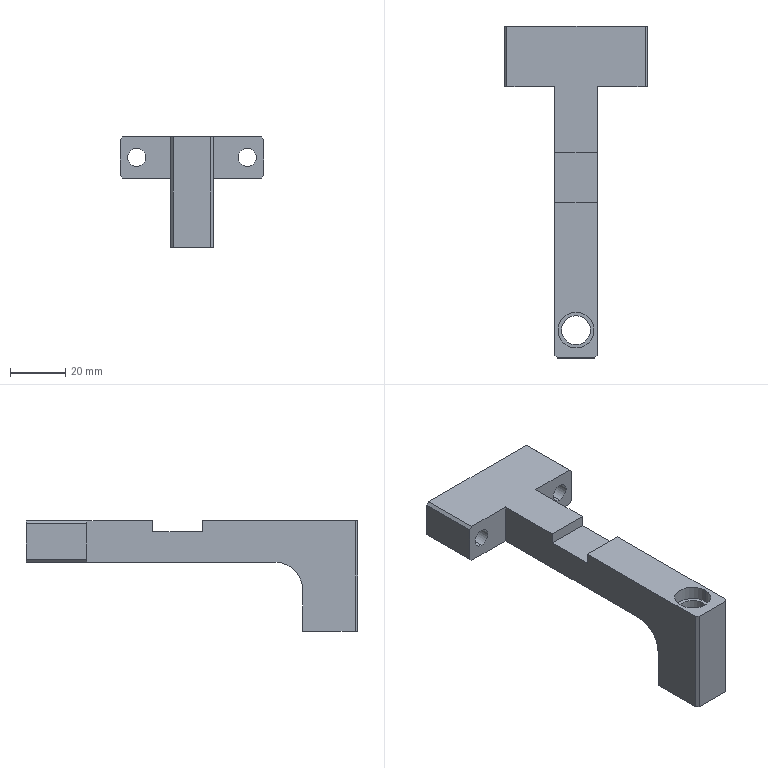Part | SolidWorks | features ICE 10, HoleWzd 3, Chamfer 1, Extrusion 1, Fillet 1, MirrorPattern 1 | 1 solid | 51 faces | box 52 x 120 x 40 mm | volume 40575 mm3 | plane 24 | cylinder 19 | cone 8 | commonest cylinder face diameters 3.3 x4 5 x4 6.6 x4 13 x4 10.5 x2 20 x1
STEP:
#1=CARTESIAN_POINT('',(-2.4,22.7,-0.35));
#2=VERTEX_POINT('',#1);
#3=CARTESIAN_POINT('',(-2.4,22.7,-3.65));
#4=VERTEX_POINT('',#3);
#5=CARTESIAN_POINT('',(-2.4,22.7,-2.));
#6=DIRECTION('',(1.,0.,0.));
#7=DIRECTION('',(0.,0.,-1.));
#8=AXIS2_PLACEMENT_3D('',#5,#6,#7);
#9=CIRCLE('',#8,1.65);
#10=EDGE_CURVE('',#2,#4,#9,.T.);
#11=ORIENTED_EDGE('',*,*,#10,.F.);
#12=CARTESIAN_POINT('',(7.7,22.7,-0.35));
#13=VERTEX_POINT('',#12);
#14=CARTESIAN_POINT('',(7.7,22.7,-0.35));
#15=DIRECTION('',(1.,0.,0.));
#16=VECTOR('',#15,1000.);
#17=LINE('',#14,#16);
#18=EDGE_CURVE('',#2,#13,#17,.T.);
#19=ORIENTED_EDGE('',*,*,#18,.T.);
#20=CARTESIAN_POINT('',(7.7,22.7,-3.65));
#21=VERTEX_POINT('',#20);
#22=CARTESIAN_POINT('',(7.7,22.7,-2.));
#23=DIRECTION('',(1.,0.,0.));
#24=DIRECTION('',(0.,0.,-1.));
#25=AXIS2_PLACEMENT_3D('',#22,#23,#24);
#26=CIRCLE('',#25,1.65);
#27=EDGE_CURVE('',#13,#21,#26,.T.);
#28=ORIENTED_EDGE('',*,*,#27,.T.);
#29=CARTESIAN_POINT('',(7.7,22.7,-3.65));
#30=DIRECTION('',(1.,0.,0.));
#31=VECTOR('',#30,1000.);
#32=LINE('',#29,#31);
#33=EDGE_CURVE('',#4,#21,#32,.T.);
#34=ORIENTED_EDGE('',*,*,#33,.F.);
#35=EDGE_LOOP('',(#11,#19,#28,#34));
#36=FACE_OUTER_BOUND('',#35,.T.);
#37=CARTESIAN_POINT('',(7.7,22.7,-2.));
#38=DIRECTION('',(1.,0.,0.));
#39=DIRECTION('',(0.,0.,-1.));
#40=AXIS2_PLACEMENT_3D('',#37,#38,#39);
#41=CYLINDRICAL_SURFACE('',#40,1.65);
#42=ADVANCED_FACE('',(#36),#41,.F.);
#43=CARTESIAN_POINT('',(-3.391,22.7,-2.));
#44=VERTEX_POINT('',#43);
#45=CARTESIAN_POINT('',(-2.4,22.7,-3.65));
#46=DIRECTION('',(0.515,0.,-0.8572));
#47=VECTOR('',#46,1000.);
#48=LINE('',#45,#47);
#49=EDGE_CURVE('',#44,#4,#48,.T.);
#50=ORIENTED_EDGE('',*,*,#49,.F.);
#51=CARTESIAN_POINT('',(-2.4,22.7,-0.35));
#52=DIRECTION('',(0.515,0.,0.8572));
#53=VECTOR('',#52,1000.);
#54=LINE('',#51,#53);
#55=EDGE_CURVE('',#44,#2,#54,.T.);
#56=ORIENTED_EDGE('',*,*,#55,.T.);
#57=ORIENTED_EDGE('',*,*,#10,.T.);
#58=EDGE_LOOP('',(#50,#56,#57));
#59=FACE_OUTER_BOUND('',#58,.T.);
#60=CARTESIAN_POINT('',(-2.4,22.7,-2.));
#61=DIRECTION('',(1.,0.,0.));
#62=DIRECTION('',(0.,0.,-1.));
#63=AXIS2_PLACEMENT_3D('',#60,#61,#62);
#64=CONICAL_SURFACE('',#63,1.65,1.03);
#65=ADVANCED_FACE('',(#59),#64,.F.);
#66=CARTESIAN_POINT('',(-2.4,-12.3,-0.35));
#67=VERTEX_POINT('',#66);
#68=CARTESIAN_POINT('',(-2.4,-12.3,-3.65));
#69=VERTEX_POINT('',#68);
#70=CARTESIAN_POINT('',(-2.4,-12.3,-2.));
#71=DIRECTION('',(1.,0.,0.));
#72=DIRECTION('',(0.,0.,-1.));
#73=AXIS2_PLACEMENT_3D('',#70,#71,#72);
#74=CIRCLE('',#73,1.65);
#75=EDGE_CURVE('',#67,#69,#74,.T.);
#76=ORIENTED_EDGE('',*,*,#75,.F.);
#77=CARTESIAN_POINT('',(7.7,-12.3,-0.35));
#78=VERTEX_POINT('',#77);
#79=CARTESIAN_POINT('',(7.7,-12.3,-0.35));
#80=DIRECTION('',(1.,0.,0.));
#81=VECTOR('',#80,1000.);
#82=LINE('',#79,#81);
#83=EDGE_CURVE('',#67,#78,#82,.T.);
#84=ORIENTED_EDGE('',*,*,#83,.T.);
#85=CARTESIAN_POINT('',(7.7,-12.3,-3.65));
#86=VERTEX_POINT('',#85);
#87=CARTESIAN_POINT('',(7.7,-12.3,-2.));
#88=DIRECTION('',(1.,0.,0.));
#89=DIRECTION('',(0.,0.,-1.));
#90=AXIS2_PLACEMENT_3D('',#87,#88,#89);
#91=CIRCLE('',#90,1.65);
#92=EDGE_CURVE('',#78,#86,#91,.T.);
#93=ORIENTED_EDGE('',*,*,#92,.T.);
#94=CARTESIAN_POINT('',(7.7,-12.3,-3.65));
#95=DIRECTION('',(1.,0.,0.));
#96=VECTOR('',#95,1000.);
#97=LINE('',#94,#96);
#98=EDGE_CURVE('',#69,#86,#97,.T.);
#99=ORIENTED_EDGE('',*,*,#98,.F.);
#100=EDGE_LOOP('',(#76,#84,#93,#99));
#101=FACE_OUTER_BOUND('',#100,.T.);
#102=CARTESIAN_POINT('',(7.7,-12.3,-2.));
#103=DIRECTION('',(1.,0.,0.));
#104=DIRECTION('',(0.,0.,-1.));
#105=AXIS2_PLACEMENT_3D('',#102,#103,#104);
#106=CYLINDRICAL_SURFACE('',#105,1.65);
#107=ADVANCED_FACE('',(#101),#106,.F.);
#108=CARTESIAN_POINT('',(-3.391,-12.3,-2.));
#109=VERTEX_POINT('',#108);
#110=CARTESIAN_POINT('',(-2.4,-12.3,-3.65));
#111=DIRECTION('',(0.515,0.,-0.8572));
#112=VECTOR('',#111,1000.);
#113=LINE('',#110,#112);
#114=EDGE_CURVE('',#109,#69,#113,.T.);
#115=ORIENTED_EDGE('',*,*,#114,.F.);
#116=CARTESIAN_POINT('',(-2.4,-12.3,-0.35));
#117=DIRECTION('',(0.515,0.,0.8572));
#118=VECTOR('',#117,1000.);
#119=LINE('',#116,#118);
#120=EDGE_CURVE('',#109,#67,#119,.T.);
#121=ORIENTED_EDGE('',*,*,#120,.T.);
#122=ORIENTED_EDGE('',*,*,#75,.T.);
#123=EDGE_LOOP('',(#115,#121,#122));
#124=FACE_OUTER_BOUND('',#123,.T.);
#125=CARTESIAN_POINT('',(-2.4,-12.3,-2.));
#126=DIRECTION('',(1.,0.,0.));
#127=DIRECTION('',(0.,0.,-1.));
#128=AXIS2_PLACEMENT_3D('',#125,#126,#127);
#129=CONICAL_SURFACE('',#128,1.65,1.03);
#130=ADVANCED_FACE('',(#124),#129,.F.);
#131=CARTESIAN_POINT('',(6.5,-50.,-27.5));
#132=VERTEX_POINT('',#131);
#133=CARTESIAN_POINT('',(-6.5,-50.,-27.5));
#134=VERTEX_POINT('',#133);
#135=CARTESIAN_POINT('',(0.,-50.,-27.5));
#136=DIRECTION('',(0.,0.,-1.));
#137=DIRECTION('',(-1.,0.,0.));
#138=AXIS2_PLACEMENT_3D('',#135,#136,#137);
#139=CIRCLE('',#138,6.5);
#140=EDGE_CURVE('',#132,#134,#139,.T.);
#141=ORIENTED_EDGE('',*,*,#140,.F.);
#142=CARTESIAN_POINT('',(6.5,-50.,-32.5));
#143=VERTEX_POINT('',#142);
#144=CARTESIAN_POINT('',(6.5,-50.,-27.5));
#145=DIRECTION('',(0.,0.,-1.));
#146=VECTOR('',#145,1000.);
#147=LINE('',#144,#146);
#148=EDGE_CURVE('',#132,#143,#147,.T.);
#149=ORIENTED_EDGE('',*,*,#148,.T.);
#150=CARTESIAN_POINT('',(-6.5,-50.,-32.5));
#151=VERTEX_POINT('',#150);
#152=CARTESIAN_POINT('',(0.,-50.,-32.5));
#153=DIRECTION('',(0.,0.,-1.));
#154=DIRECTION('',(-1.,0.,0.));
#155=AXIS2_PLACEMENT_3D('',#152,#153,#154);
#156=CIRCLE('',#155,6.5);
#157=EDGE_CURVE('',#143,#151,#156,.T.);
#158=ORIENTED_EDGE('',*,*,#157,.T.);
#159=CARTESIAN_POINT('',(-6.5,-50.,-27.5));
#160=DIRECTION('',(0.,0.,-1.));
#161=VECTOR('',#160,1000.);
#162=LINE('',#159,#161);
#163=EDGE_CURVE('',#134,#151,#162,.T.);
#164=ORIENTED_EDGE('',*,*,#163,.F.);
#165=EDGE_LOOP('',(#141,#149,#158,#164));
#166=FACE_OUTER_BOUND('',#165,.T.);
#167=CARTESIAN_POINT('',(0.,-50.,-27.5));
#168=DIRECTION('',(0.,0.,-1.));
#169=DIRECTION('',(-1.,0.,0.));
#170=AXIS2_PLACEMENT_3D('',#167,#168,#169);
#171=CYLINDRICAL_SURFACE('',#170,6.5);
#172=ADVANCED_FACE('',(#166),#171,.F.);
#173=CARTESIAN_POINT('',(-6.5,-50.,2.5));
#174=VERTEX_POINT('',#173);
#175=CARTESIAN_POINT('',(6.5,-50.,2.5));
#176=VERTEX_POINT('',#175);
#177=CARTESIAN_POINT('',(0.,-50.,2.5));
#178=DIRECTION('',(0.,0.,1.));
#179=DIRECTION('',(1.,0.,0.));
#180=AXIS2_PLACEMENT_3D('',#177,#178,#179);
#181=CIRCLE('',#180,6.5);
#182=EDGE_CURVE('',#174,#176,#181,.T.);
#183=ORIENTED_EDGE('',*,*,#182,.F.);
#184=CARTESIAN_POINT('',(-6.5,-50.,7.5));
#185=VERTEX_POINT('',#184);
#186=CARTESIAN_POINT('',(-6.5,-50.,2.5));
#187=DIRECTION('',(0.,0.,1.));
#188=VECTOR('',#187,1000.);
#189=LINE('',#186,#188);
#190=EDGE_CURVE('',#174,#185,#189,.T.);
#191=ORIENTED_EDGE('',*,*,#190,.T.);
#192=CARTESIAN_POINT('',(6.5,-50.,7.5));
#193=VERTEX_POINT('',#192);
#194=CARTESIAN_POINT('',(0.,-50.,7.5));
#195=DIRECTION('',(0.,0.,1.));
#196=DIRECTION('',(1.,0.,0.));
#197=AXIS2_PLACEMENT_3D('',#194,#195,#196);
#198=CIRCLE('',#197,6.5);
#199=EDGE_CURVE('',#185,#193,#198,.T.);
#200=ORIENTED_EDGE('',*,*,#199,.T.);
#201=CARTESIAN_POINT('',(6.5,-50.,2.5));
#202=DIRECTION('',(0.,0.,1.));
#203=VECTOR('',#202,1000.);
#204=LINE('',#201,#203);
#205=EDGE_CURVE('',#176,#193,#204,.T.);
#206=ORIENTED_EDGE('',*,*,#205,.F.);
#207=EDGE_LOOP('',(#183,#191,#200,#206));
#208=FACE_OUTER_BOUND('',#207,.T.);
#209=CARTESIAN_POINT('',(0.,-50.,2.5));
#210=DIRECTION('',(0.,0.,1.));
#211=DIRECTION('',(1.,0.,0.));
#212=AXIS2_PLACEMENT_3D('',#209,#210,#211);
#213=CYLINDRICAL_SURFACE('',#212,6.5);
#214=ADVANCED_FACE('',(#208),#213,.F.);
#215=CARTESIAN_POINT('',(-10.,49.,-2.5));
#216=VERTEX_POINT('',#215);
#217=CARTESIAN_POINT('',(-10.,49.,2.5));
#218=VERTEX_POINT('',#217);
#219=CARTESIAN_POINT('',(-10.,49.,0.));
#220=DIRECTION('',(0.,1.,0.));
#221=DIRECTION('',(0.,0.,1.));
#222=AXIS2_PLACEMENT_3D('',#219,#220,#221);
#223=CIRCLE('',#222,2.5);
#224=EDGE_CURVE('',#216,#218,#223,.T.);
#225=ORIENTED_EDGE('',*,*,#224,.F.);
#226=CARTESIAN_POINT('',(-10.,60.,-2.5));
#227=VERTEX_POINT('',#226);
#228=CARTESIAN_POINT('',(-10.,60.,-2.5));
#229=DIRECTION('',(0.,1.,0.));
#230=VECTOR('',#229,1000.);
#231=LINE('',#228,#230);
#232=EDGE_CURVE('',#216,#227,#231,.T.);
#233=ORIENTED_EDGE('',*,*,#232,.T.);
#234=CARTESIAN_POINT('',(-10.,60.,2.5));
#235=VERTEX_POINT('',#234);
#236=CARTESIAN_POINT('',(-10.,60.,0.));
#237=DIRECTION('',(0.,1.,0.));
#238=DIRECTION('',(0.,0.,1.));
#239=AXIS2_PLACEMENT_3D('',#236,#237,#238);
#240=CIRCLE('',#239,2.5);
#241=EDGE_CURVE('',#227,#235,#240,.T.);
#242=ORIENTED_EDGE('',*,*,#241,.T.);
#243=CARTESIAN_POINT('',(-10.,60.,2.5));
#244=DIRECTION('',(0.,1.,0.));
#245=VECTOR('',#244,1000.);
#246=LINE('',#243,#245);
#247=EDGE_CURVE('',#218,#235,#246,.T.);
#248=ORIENTED_EDGE('',*,*,#247,.F.);
#249=EDGE_LOOP('',(#225,#233,#242,#248));
#250=FACE_OUTER_BOUND('',#249,.T.);
#251=CARTESIAN_POINT('',(-10.,60.,0.));
#252=DIRECTION('',(0.,1.,0.));
#253=DIRECTION('',(0.,0.,1.));
#254=AXIS2_PLACEMENT_3D('',#251,#252,#253);
#255=CYLINDRICAL_SURFACE('',#254,2.5);
#256=ADVANCED_FACE('',(#250),#255,.F.);
#257=CARTESIAN_POINT('',(-10.,47.498,0.));
#258=VERTEX_POINT('',#257);
#259=CARTESIAN_POINT('',(-10.,49.,2.5));
#260=DIRECTION('',(0.,0.515,0.8572));
#261=VECTOR('',#260,1000.);
#262=LINE('',#259,#261);
#263=EDGE_CURVE('',#258,#218,#262,.T.);
#264=ORIENTED_EDGE('',*,*,#263,.F.);
#265=CARTESIAN_POINT('',(-10.,49.,-2.5));
#266=DIRECTION('',(0.,0.515,-0.8572));
#267=VECTOR('',#266,1000.);
#268=LINE('',#265,#267);
#269=EDGE_CURVE('',#258,#216,#268,.T.);
#270=ORIENTED_EDGE('',*,*,#269,.T.);
#271=ORIENTED_EDGE('',*,*,#224,.T.);
#272=EDGE_LOOP('',(#264,#270,#271));
#273=FACE_OUTER_BOUND('',#272,.T.);
#274=CARTESIAN_POINT('',(-10.,49.,0.));
#275=DIRECTION('',(0.,1.,0.));
#276=DIRECTION('',(0.,0.,1.));
#277=AXIS2_PLACEMENT_3D('',#274,#275,#276);
#278=CONICAL_SURFACE('',#277,2.5,1.03);
#279=ADVANCED_FACE('',(#273),#278,.F.);
#280=CARTESIAN_POINT('',(10.,49.,-2.5));
#281=VERTEX_POINT('',#280);
#282=CARTESIAN_POINT('',(10.,49.,2.5));
#283=VERTEX_POINT('',#282);
#284=CARTESIAN_POINT('',(10.,49.,0.));
#285=DIRECTION('',(0.,1.,0.));
#286=DIRECTION('',(0.,0.,1.));
#287=AXIS2_PLACEMENT_3D('',#284,#285,#286);
#288=CIRCLE('',#287,2.5);
#289=EDGE_CURVE('',#281,#283,#288,.T.);
#290=ORIENTED_EDGE('',*,*,#289,.F.);
#291=CARTESIAN_POINT('',(10.,60.,-2.5));
#292=VERTEX_POINT('',#291);
#293=CARTESIAN_POINT('',(10.,60.,-2.5));
#294=DIRECTION('',(0.,1.,0.));
#295=VECTOR('',#294,1000.);
#296=LINE('',#293,#295);
#297=EDGE_CURVE('',#281,#292,#296,.T.);
#298=ORIENTED_EDGE('',*,*,#297,.T.);
#299=CARTESIAN_POINT('',(10.,60.,2.5));
#300=VERTEX_POINT('',#299);
#301=CARTESIAN_POINT('',(10.,60.,0.));
#302=DIRECTION('',(0.,1.,0.));
#303=DIRECTION('',(0.,0.,1.));
#304=AXIS2_PLACEMENT_3D('',#301,#302,#303);
#305=CIRCLE('',#304,2.5);
#306=EDGE_CURVE('',#292,#300,#305,.T.);
#307=ORIENTED_EDGE('',*,*,#306,.T.);
#308=CARTESIAN_POINT('',(10.,60.,2.5));
#309=DIRECTION('',(0.,1.,0.));
#310=VECTOR('',#309,1000.);
#311=LINE('',#308,#310);
#312=EDGE_CURVE('',#283,#300,#311,.T.);
#313=ORIENTED_EDGE('',*,*,#312,.F.);
#314=EDGE_LOOP('',(#290,#298,#307,#313));
#315=FACE_OUTER_BOUND('',#314,.T.);
#316=CARTESIAN_POINT('',(10.,60.,0.));
#317=DIRECTION('',(0.,1.,0.));
#318=DIRECTION('',(0.,0.,1.));
#319=AXIS2_PLACEMENT_3D('',#316,#317,#318);
#320=CYLINDRICAL_SURFACE('',#319,2.5);
#321=ADVANCED_FACE('',(#315),#320,.F.);
#322=CARTESIAN_POINT('',(10.,47.498,0.));
#323=VERTEX_POINT('',#322);
#324=CARTESIAN_POINT('',(10.,49.,2.5));
#325=DIRECTION('',(0.,0.515,0.8572));
#326=VECTOR('',#325,1000.);
#327=LINE('',#324,#326);
#328=EDGE_CURVE('',#323,#283,#327,.T.);
#329=ORIENTED_EDGE('',*,*,#328,.F.);
#330=CARTESIAN_POINT('',(10.,49.,-2.5));
#331=DIRECTION('',(0.,0.515,-0.8572));
#332=VECTOR('',#331,1000.);
#333=LINE('',#330,#332);
#334=EDGE_CURVE('',#323,#281,#333,.T.);
#335=ORIENTED_EDGE('',*,*,#334,.T.);
#336=ORIENTED_EDGE('',*,*,#289,.T.);
#337=EDGE_LOOP('',(#329,#335,#336));
#338=FACE_OUTER_BOUND('',#337,.T.);
#339=CARTESIAN_POINT('',(10.,49.,0.));
#340=DIRECTION('',(0.,1.,0.));
#341=DIRECTION('',(0.,0.,1.));
#342=AXIS2_PLACEMENT_3D('',#339,#340,#341);
#343=CONICAL_SURFACE('',#342,2.5,1.03);
#344=ADVANCED_FACE('',(#338),#343,.F.);
#345=CARTESIAN_POINT('',(-20.,38.,-3.3));
#346=VERTEX_POINT('',#345);
#347=CARTESIAN_POINT('',(-20.,38.,3.3));
#348=VERTEX_POINT('',#347);
#349=CARTESIAN_POINT('',(-20.,38.,0.));
#350=DIRECTION('',(0.,1.,0.));
#351=DIRECTION('',(0.,0.,1.));
#352=AXIS2_PLACEMENT_3D('',#349,#350,#351);
#353=CIRCLE('',#352,3.3);
#354=EDGE_CURVE('',#346,#348,#353,.T.);
#355=ORIENTED_EDGE('',*,*,#354,.F.);
#356=CARTESIAN_POINT('',(-20.,60.,-3.3));
#357=VERTEX_POINT('',#356);
#358=CARTESIAN_POINT('',(-20.,60.,-3.3));
#359=DIRECTION('',(0.,1.,0.));
#360=VECTOR('',#359,1000.);
#361=LINE('',#358,#360);
#362=EDGE_CURVE('',#346,#357,#361,.T.);
#363=ORIENTED_EDGE('',*,*,#362,.T.);
#364=CARTESIAN_POINT('',(-20.,60.,3.3));
#365=VERTEX_POINT('',#364);
#366=CARTESIAN_POINT('',(-20.,60.,0.));
#367=DIRECTION('',(0.,1.,0.));
#368=DIRECTION('',(0.,0.,1.));
#369=AXIS2_PLACEMENT_3D('',#366,#367,#368);
#370=CIRCLE('',#369,3.3);
#371=EDGE_CURVE('',#357,#365,#370,.T.);
#372=ORIENTED_EDGE('',*,*,#371,.T.);
#373=CARTESIAN_POINT('',(-20.,60.,3.3));
#374=DIRECTION('',(0.,1.,0.));
#375=VECTOR('',#374,1000.);
#376=LINE('',#373,#375);
#377=EDGE_CURVE('',#348,#365,#376,.T.);
#378=ORIENTED_EDGE('',*,*,#377,.F.);
#379=EDGE_LOOP('',(#355,#363,#372,#378));
#380=FACE_OUTER_BOUND('',#379,.T.);
#381=CARTESIAN_POINT('',(-20.,60.,0.));
#382=DIRECTION('',(0.,1.,0.));
#383=DIRECTION('',(0.,0.,1.));
#384=AXIS2_PLACEMENT_3D('',#381,#382,#383);
#385=CYLINDRICAL_SURFACE('',#384,3.3);
#386=ADVANCED_FACE('',(#380),#385,.F.);
#387=CARTESIAN_POINT('',(20.,38.,3.3));
#388=VERTEX_POINT('',#387);
#389=CARTESIAN_POINT('',(20.,38.,-3.3));
#390=VERTEX_POINT('',#389);
#391=CARTESIAN_POINT('',(20.,38.,0.));
#392=DIRECTION('',(0.,-1.,0.));
#393=DIRECTION('',(0.,0.,-1.));
#394=AXIS2_PLACEMENT_3D('',#391,#392,#393);
#395=CIRCLE('',#394,3.3);
#396=EDGE_CURVE('',#388,#390,#395,.T.);
#397=ORIENTED_EDGE('',*,*,#396,.T.);
#398=CARTESIAN_POINT('',(20.,60.,-3.3));
#399=VERTEX_POINT('',#398);
#400=CARTESIAN_POINT('',(20.,60.,-3.3));
#401=DIRECTION('',(0.,1.,0.));
#402=VECTOR('',#401,1000.);
#403=LINE('',#400,#402);
#404=EDGE_CURVE('',#390,#399,#403,.T.);
#405=ORIENTED_EDGE('',*,*,#404,.T.);
#406=CARTESIAN_POINT('',(20.,60.,3.3));
#407=VERTEX_POINT('',#406);
#408=CARTESIAN_POINT('',(20.,60.,0.));
#409=DIRECTION('',(0.,1.,0.));
#410=DIRECTION('',(0.,0.,1.));
#411=AXIS2_PLACEMENT_3D('',#408,#409,#410);
#412=CIRCLE('',#411,3.3);
#413=EDGE_CURVE('',#399,#407,#412,.T.);
#414=ORIENTED_EDGE('',*,*,#413,.T.);
#415=CARTESIAN_POINT('',(20.,60.,3.3));
#416=DIRECTION('',(0.,1.,0.));
#417=VECTOR('',#416,1000.);
#418=LINE('',#415,#417);
#419=EDGE_CURVE('',#388,#407,#418,.T.);
#420=ORIENTED_EDGE('',*,*,#419,.F.);
#421=EDGE_LOOP('',(#397,#405,#414,#420));
#422=FACE_OUTER_BOUND('',#421,.T.);
#423=CARTESIAN_POINT('',(20.,60.,0.));
#424=DIRECTION('',(0.,1.,0.));
#425=DIRECTION('',(0.,0.,1.));
#426=AXIS2_PLACEMENT_3D('',#423,#424,#425);
#427=CYLINDRICAL_SURFACE('',#426,3.3);
#428=ADVANCED_FACE('',(#422),#427,.F.);
#429=CARTESIAN_POINT('',(-5.25,-50.,-27.5));
#430=VERTEX_POINT('',#429);
#431=CARTESIAN_POINT('',(5.25,-50.,-27.5));
#432=VERTEX_POINT('',#431);
#433=CARTESIAN_POINT('',(0.,-50.,-27.5));
#434=DIRECTION('',(0.,0.,1.));
#435=DIRECTION('',(-1.,0.,0.));
#436=AXIS2_PLACEMENT_3D('',#433,#434,#435);
#437=CIRCLE('',#436,5.25);
#438=EDGE_CURVE('',#430,#432,#437,.T.);
#439=ORIENTED_EDGE('',*,*,#438,.F.);
#440=CARTESIAN_POINT('',(-5.25,-50.,2.5));
#441=VERTEX_POINT('',#440);
#442=CARTESIAN_POINT('',(-5.25,-50.,-32.5));
#443=DIRECTION('',(0.,0.,1.));
#444=VECTOR('',#443,1000.);
#445=LINE('',#442,#444);
#446=EDGE_CURVE('',#430,#441,#445,.T.);
#447=ORIENTED_EDGE('',*,*,#446,.T.);
#448=CARTESIAN_POINT('',(5.25,-50.,2.5));
#449=VERTEX_POINT('',#448);
#450=CARTESIAN_POINT('',(0.,-50.,2.5));
#451=DIRECTION('',(0.,0.,-1.));
#452=DIRECTION('',(1.,0.,0.));
#453=AXIS2_PLACEMENT_3D('',#450,#451,#452);
#454=CIRCLE('',#453,5.25);
#455=EDGE_CURVE('',#449,#441,#454,.T.);
#456=ORIENTED_EDGE('',*,*,#455,.F.);
#457=CARTESIAN_POINT('',(5.25,-50.,-32.5));
#458=DIRECTION('',(0.,0.,1.));
#459=VECTOR('',#458,1000.);
#460=LINE('',#457,#459);
#461=EDGE_CURVE('',#432,#449,#460,.T.);
#462=ORIENTED_EDGE('',*,*,#461,.F.);
#463=EDGE_LOOP('',(#439,#447,#456,#462));
#464=FACE_OUTER_BOUND('',#463,.T.);
#465=CARTESIAN_POINT('',(0.,-50.,-32.5));
#466=DIRECTION('',(0.,0.,1.));
#467=DIRECTION('',(1.,0.,0.));
#468=AXIS2_PLACEMENT_3D('',#465,#466,#467);
#469=CYLINDRICAL_SURFACE('',#468,5.25);
#470=ADVANCED_FACE('',(#464),#469,.F.);
#471=CARTESIAN_POINT('',(-7.7,14.2,7.5));
#472=VERTEX_POINT('',#471);
#473=CARTESIAN_POINT('',(7.7,14.2,7.5));
#474=VERTEX_POINT('',#473);
#475=CARTESIAN_POINT('',(-26.,14.2,7.5));
#476=DIRECTION('',(1.,0.,0.));
#477=VECTOR('',#476,1000.);
#478=LINE('',#475,#477);
#479=EDGE_CURVE('',#472,#474,#478,.T.);
#480=ORIENTED_EDGE('',*,*,#479,.T.);
#481=CARTESIAN_POINT('',(7.7,38.,7.5));
#482=VERTEX_POINT('',#481);
#483=CARTESIAN_POINT('',(7.7,38.,7.5));
#484=DIRECTION('',(0.,1.,0.));
#485=VECTOR('',#484,1000.);
#486=LINE('',#483,#485);
#487=EDGE_CURVE('',#474,#482,#486,.T.);
#488=ORIENTED_EDGE('',*,*,#487,.T.);
#489=CARTESIAN_POINT('',(25.,38.,7.5));
#490=VERTEX_POINT('',#489);
#491=CARTESIAN_POINT('',(26.,38.,7.5));
#492=DIRECTION('',(1.,0.,0.));
#493=VECTOR('',#492,1000.);
#494=LINE('',#491,#493);
#495=EDGE_CURVE('',#482,#490,#494,.T.);
#496=ORIENTED_EDGE('',*,*,#495,.T.);
#497=CARTESIAN_POINT('',(25.,60.,7.5));
#498=VERTEX_POINT('',#497);
#499=CARTESIAN_POINT('',(25.,60.,7.5));
#500=DIRECTION('',(0.,1.,0.));
#501=VECTOR('',#500,1000.);
#502=LINE('',#499,#501);
#503=EDGE_CURVE('',#490,#498,#502,.T.);
#504=ORIENTED_EDGE('',*,*,#503,.T.);
#505=CARTESIAN_POINT('',(-25.,60.,7.5));
#506=VERTEX_POINT('',#505);
#507=CARTESIAN_POINT('',(-26.,60.,7.5));
#508=DIRECTION('',(-1.,0.,0.));
#509=VECTOR('',#508,1000.);
#510=LINE('',#507,#509);
#511=EDGE_CURVE('',#498,#506,#510,.T.);
#512=ORIENTED_EDGE('',*,*,#511,.T.);
#513=CARTESIAN_POINT('',(-25.,38.,7.5));
#514=VERTEX_POINT('',#513);
#515=CARTESIAN_POINT('',(-25.,38.,7.5));
#516=DIRECTION('',(0.,-1.,0.));
#517=VECTOR('',#516,1000.);
#518=LINE('',#515,#517);
#519=EDGE_CURVE('',#506,#514,#518,.T.);
#520=ORIENTED_EDGE('',*,*,#519,.T.);
#521=CARTESIAN_POINT('',(-7.7,38.,7.5));
#522=VERTEX_POINT('',#521);
#523=CARTESIAN_POINT('',(-26.,38.,7.5));
#524=DIRECTION('',(-1.,0.,0.));
#525=VECTOR('',#524,1000.);
#526=LINE('',#523,#525);
#527=EDGE_CURVE('',#522,#514,#526,.T.);
#528=ORIENTED_EDGE('',*,*,#527,.F.);
#529=CARTESIAN_POINT('',(-7.7,38.,7.5));
#530=DIRECTION('',(0.,1.,0.));
#531=VECTOR('',#530,1000.);
#532=LINE('',#529,#531);
#533=EDGE_CURVE('',#472,#522,#532,.T.);
#534=ORIENTED_EDGE('',*,*,#533,.F.);
#535=EDGE_LOOP('',(#480,#488,#496,#504,#512,#520,#528,#534));
#536=FACE_OUTER_BOUND('',#535,.T.);
#537=CARTESIAN_POINT('',(0.,0.,7.5));
#538=DIRECTION('',(0.,0.,1.));
#539=DIRECTION('',(1.,0.,0.));
#540=AXIS2_PLACEMENT_3D('',#537,#538,#539);
#541=PLANE('',#540);
#542=ADVANCED_FACE('',(#536),#541,.T.);
#543=ORIENTED_EDGE('',*,*,#446,.F.);
#544=CARTESIAN_POINT('',(0.,-50.,-27.5));
#545=DIRECTION('',(0.,0.,1.));
#546=DIRECTION('',(-1.,0.,0.));
#547=AXIS2_PLACEMENT_3D('',#544,#545,#546);
#548=CIRCLE('',#547,5.25);
#549=EDGE_CURVE('',#432,#430,#548,.T.);
#550=ORIENTED_EDGE('',*,*,#549,.F.);
#551=ORIENTED_EDGE('',*,*,#461,.T.);
#552=CARTESIAN_POINT('',(0.,-50.,2.5));
#553=DIRECTION('',(0.,0.,-1.));
#554=DIRECTION('',(1.,0.,0.));
#555=AXIS2_PLACEMENT_3D('',#552,#553,#554);
#556=CIRCLE('',#555,5.25);
#557=EDGE_CURVE('',#441,#449,#556,.T.);
#558=ORIENTED_EDGE('',*,*,#557,.F.);
#559=EDGE_LOOP('',(#543,#550,#551,#558));
#560=FACE_OUTER_BOUND('',#559,.T.);
#561=CARTESIAN_POINT('',(0.,-50.,-32.5));
#562=DIRECTION('',(0.,0.,1.));
#563=DIRECTION('',(1.,0.,0.));
#564=AXIS2_PLACEMENT_3D('',#561,#562,#563);
#565=CYLINDRICAL_SURFACE('',#564,5.25);
#566=ADVANCED_FACE('',(#560),#565,.F.);
#567=CARTESIAN_POINT('',(7.7,-30.,-7.5));
#568=VERTEX_POINT('',#567);
#569=CARTESIAN_POINT('',(7.7,38.,-7.5));
#570=VERTEX_POINT('',#569);
#571=CARTESIAN_POINT('',(7.7,38.,-7.5));
#572=DIRECTION('',(0.,1.,0.));
#573=VECTOR('',#572,1000.);
#574=LINE('',#571,#573);
#575=EDGE_CURVE('',#568,#570,#574,.T.);
#576=ORIENTED_EDGE('',*,*,#575,.F.);
#577=CARTESIAN_POINT('',(-7.7,-30.,-7.5));
#578=VERTEX_POINT('',#577);
#579=CARTESIAN_POINT('',(-7.7,-30.,-7.5));
#580=DIRECTION('',(-1.,0.,0.));
#581=VECTOR('',#580,1000.);
#582=LINE('',#579,#581);
#583=EDGE_CURVE('',#568,#578,#582,.T.);
#584=ORIENTED_EDGE('',*,*,#583,.T.);
#585=CARTESIAN_POINT('',(-7.7,38.,-7.5));
#586=VERTEX_POINT('',#585);
#587=CARTESIAN_POINT('',(-7.7,38.,-7.5));
#588=DIRECTION('',(0.,1.,0.));
#589=VECTOR('',#588,1000.);
#590=LINE('',#587,#589);
#591=EDGE_CURVE('',#578,#586,#590,.T.);
#592=ORIENTED_EDGE('',*,*,#591,.T.);
#593=CARTESIAN_POINT('',(-25.,38.,-7.5));
#594=VERTEX_POINT('',#593);
#595=CARTESIAN_POINT('',(-26.,38.,-7.5));
#596=DIRECTION('',(-1.,0.,0.));
#597=VECTOR('',#596,1000.);
#598=LINE('',#595,#597);
#599=EDGE_CURVE('',#586,#594,#598,.T.);
#600=ORIENTED_EDGE('',*,*,#599,.T.);
#601=CARTESIAN_POINT('',(-25.,60.,-7.5));
#602=VERTEX_POINT('',#601);
#603=CARTESIAN_POINT('',(-25.,0.,-7.5));
#604=DIRECTION('',(0.,1.,0.));
#605=VECTOR('',#604,1000.);
#606=LINE('',#603,#605);
#607=EDGE_CURVE('',#594,#602,#606,.T.);
#608=ORIENTED_EDGE('',*,*,#607,.T.);
#609=CARTESIAN_POINT('',(25.,60.,-7.5));
#610=VERTEX_POINT('',#609);
#611=CARTESIAN_POINT('',(-26.,60.,-7.5));
#612=DIRECTION('',(-1.,0.,0.));
#613=VECTOR('',#612,1000.);
#614=LINE('',#611,#613);
#615=EDGE_CURVE('',#610,#602,#614,.T.);
#616=ORIENTED_EDGE('',*,*,#615,.F.);
#617=CARTESIAN_POINT('',(25.,38.,-7.5));
#618=VERTEX_POINT('',#617);
#619=CARTESIAN_POINT('',(25.,0.,-7.5));
#620=DIRECTION('',(0.,-1.,0.));
#621=VECTOR('',#620,1000.);
#622=LINE('',#619,#621);
#623=EDGE_CURVE('',#610,#618,#622,.T.);
#624=ORIENTED_EDGE('',*,*,#623,.T.);
#625=CARTESIAN_POINT('',(26.,38.,-7.5));
#626=DIRECTION('',(1.,0.,0.));
#627=VECTOR('',#626,1000.);
#628=LINE('',#625,#627);
#629=EDGE_CURVE('',#570,#618,#628,.T.);
#630=ORIENTED_EDGE('',*,*,#629,.F.);
#631=EDGE_LOOP('',(#576,#584,#592,#600,#608,#616,#624,#630));
#632=FACE_OUTER_BOUND('',#631,.T.);
#633=CARTESIAN_POINT('',(0.,0.,-7.5));
#634=DIRECTION('',(0.,0.,1.));
#635=DIRECTION('',(1.,0.,0.));
#636=AXIS2_PLACEMENT_3D('',#633,#634,#635);
#637=PLANE('',#636);
#638=ADVANCED_FACE('',(#632),#637,.F.);
#639=CARTESIAN_POINT('',(26.,38.,-6.5));
#640=VERTEX_POINT('',#639);
#641=CARTESIAN_POINT('',(26.,38.,6.5));
#642=VERTEX_POINT('',#641);
#643=CARTESIAN_POINT('',(26.,38.,-7.5));
#644=DIRECTION('',(0.,0.,1.));
#645=VECTOR('',#644,1000.);
#646=LINE('',#643,#645);
#647=EDGE_CURVE('',#640,#642,#646,.T.);
#648=ORIENTED_EDGE('',*,*,#647,.F.);
#649=CARTESIAN_POINT('',(26.,60.,-6.5));
#650=VERTEX_POINT('',#649);
#651=CARTESIAN_POINT('',(26.,60.,-6.5));
#652=DIRECTION('',(0.,1.,0.));
#653=VECTOR('',#652,1000.);
#654=LINE('',#651,#653);
#655=EDGE_CURVE('',#640,#650,#654,.T.);
#656=ORIENTED_EDGE('',*,*,#655,.T.);
#657=CARTESIAN_POINT('',(26.,60.,6.5));
#658=VERTEX_POINT('',#657);
#659=CARTESIAN_POINT('',(26.,60.,7.5));
#660=DIRECTION('',(0.,0.,-1.));
#661=VECTOR('',#660,1000.);
#662=LINE('',#659,#661);
#663=EDGE_CURVE('',#658,#650,#662,.T.);
#664=ORIENTED_EDGE('',*,*,#663,.F.);
#665=CARTESIAN_POINT('',(26.,38.,6.5));
#666=DIRECTION('',(0.,-1.,0.));
#667=VECTOR('',#666,1000.);
#668=LINE('',#665,#667);
#669=EDGE_CURVE('',#658,#642,#668,.T.);
#670=ORIENTED_EDGE('',*,*,#669,.T.);
#671=EDGE_LOOP('',(#648,#656,#664,#670));
#672=FACE_OUTER_BOUND('',#671,.T.);
#673=CARTESIAN_POINT('',(26.,60.,7.5));
#674=DIRECTION('',(-1.,0.,0.));
#675=DIRECTION('',(0.,-1.,0.));
#676=AXIS2_PLACEMENT_3D('',#673,#674,#675);
#677=PLANE('',#676);
#678=ADVANCED_FACE('',(#672),#677,.F.);
#679=CARTESIAN_POINT('',(-6.7,-60.,7.5));
#680=VERTEX_POINT('',#679);
#681=CARTESIAN_POINT('',(-6.7,-60.,-32.5));
#682=VERTEX_POINT('',#681);
#683=CARTESIAN_POINT('',(-6.7,-60.,7.5));
#684=DIRECTION('',(0.,0.,-1.));
#685=VECTOR('',#684,1000.);
#686=LINE('',#683,#685);
#687=EDGE_CURVE('',#680,#682,#686,.T.);
#688=ORIENTED_EDGE('',*,*,#687,.T.);
#689=CARTESIAN_POINT('',(6.7,-60.,-32.5));
#690=VERTEX_POINT('',#689);
#691=CARTESIAN_POINT('',(-6.7,-60.,-32.5));
#692=DIRECTION('',(-1.,0.,0.));
#693=VECTOR('',#692,1000.);
#694=LINE('',#691,#693);
#695=EDGE_CURVE('',#690,#682,#694,.T.);
#696=ORIENTED_EDGE('',*,*,#695,.F.);
#697=CARTESIAN_POINT('',(6.7,-60.,7.5));
#698=VERTEX_POINT('',#697);
#699=CARTESIAN_POINT('',(6.7,-60.,7.5));
#700=DIRECTION('',(0.,0.,1.));
#701=VECTOR('',#700,1000.);
#702=LINE('',#699,#701);
#703=EDGE_CURVE('',#690,#698,#702,.T.);
#704=ORIENTED_EDGE('',*,*,#703,.T.);
#705=CARTESIAN_POINT('',(-26.,-60.,7.5));
#706=DIRECTION('',(1.,0.,0.));
#707=VECTOR('',#706,1000.);
#708=LINE('',#705,#707);
#709=EDGE_CURVE('',#680,#698,#708,.T.);
#710=ORIENTED_EDGE('',*,*,#709,.F.);
#711=EDGE_LOOP('',(#688,#696,#704,#710));
#712=FACE_OUTER_BOUND('',#711,.T.);
#713=CARTESIAN_POINT('',(-26.,-60.,7.5));
#714=DIRECTION('',(0.,1.,0.));
#715=DIRECTION('',(0.,0.,1.));
#716=AXIS2_PLACEMENT_3D('',#713,#714,#715);
#717=PLANE('',#716);
#718=ADVANCED_FACE('',(#712),#717,.F.);
#719=CARTESIAN_POINT('',(-7.7,-3.8,7.5));
#720=VERTEX_POINT('',#719);
#721=CARTESIAN_POINT('',(7.7,-3.8,7.5));
#722=VERTEX_POINT('',#721);
#723=CARTESIAN_POINT('',(-26.,-3.8,7.5));
#724=DIRECTION('',(1.,0.,0.));
#725=VECTOR('',#724,1000.);
#726=LINE('',#723,#725);
#727=EDGE_CURVE('',#720,#722,#726,.T.);
#728=ORIENTED_EDGE('',*,*,#727,.F.);
#729=CARTESIAN_POINT('',(-7.7,-59.,7.5));
#730=VERTEX_POINT('',#729);
#731=CARTESIAN_POINT('',(-7.7,38.,7.5));
#732=DIRECTION('',(0.,1.,0.));
#733=VECTOR('',#732,1000.);
#734=LINE('',#731,#733);
#735=EDGE_CURVE('',#730,#720,#734,.T.);
#736=ORIENTED_EDGE('',*,*,#735,.F.);
#737=CARTESIAN_POINT('',(-33.35,-33.35,7.5));
#738=DIRECTION('',(0.7071,-0.7071,0.));
#739=VECTOR('',#738,1000.);
#740=LINE('',#737,#739);
#741=EDGE_CURVE('',#730,#680,#740,.T.);
#742=ORIENTED_EDGE('',*,*,#741,.T.);
#743=ORIENTED_EDGE('',*,*,#709,.T.);
#744=CARTESIAN_POINT('',(7.7,-59.,7.5));
#745=VERTEX_POINT('',#744);
#746=CARTESIAN_POINT('',(33.35,-33.35,7.5));
#747=DIRECTION('',(0.7071,0.7071,0.));
#748=VECTOR('',#747,1000.);
#749=LINE('',#746,#748);
#750=EDGE_CURVE('',#698,#745,#749,.T.);
#751=ORIENTED_EDGE('',*,*,#750,.T.);
#752=CARTESIAN_POINT('',(7.7,38.,7.5));
#753=DIRECTION('',(0.,1.,0.));
#754=VECTOR('',#753,1000.);
#755=LINE('',#752,#754);
#756=EDGE_CURVE('',#745,#722,#755,.T.);
#757=ORIENTED_EDGE('',*,*,#756,.T.);
#758=EDGE_LOOP('',(#728,#736,#742,#743,#751,#757));
#759=FACE_OUTER_BOUND('',#758,.T.);
#760=CARTESIAN_POINT('',(0.,-50.,7.5));
#761=DIRECTION('',(0.,0.,1.));
#762=DIRECTION('',(1.,0.,0.));
#763=AXIS2_PLACEMENT_3D('',#760,#761,#762);
#764=CIRCLE('',#763,6.5);
#765=EDGE_CURVE('',#193,#185,#764,.T.);
#766=ORIENTED_EDGE('',*,*,#765,.F.);
#767=ORIENTED_EDGE('',*,*,#199,.F.);
#768=EDGE_LOOP('',(#766,#767));
#769=FACE_BOUND('',#768,.T.);
#770=CARTESIAN_POINT('',(0.,0.,7.5));
#771=DIRECTION('',(0.,0.,1.));
#772=DIRECTION('',(1.,0.,0.));
#773=AXIS2_PLACEMENT_3D('',#770,#771,#772);
#774=PLANE('',#773);
#775=ADVANCED_FACE('',(#759,#769),#774,.T.);
#776=CARTESIAN_POINT('',(-10.,60.,0.));
#777=DIRECTION('',(0.,1.,0.));
#778=DIRECTION('',(0.,0.,1.));
#779=AXIS2_PLACEMENT_3D('',#776,#777,#778);
#780=CIRCLE('',#779,2.5);
#781=EDGE_CURVE('',#235,#227,#780,.T.);
#782=ORIENTED_EDGE('',*,*,#781,.F.);
#783=ORIENTED_EDGE('',*,*,#241,.F.);
#784=EDGE_LOOP('',(#782,#783));
#785=FACE_BOUND('',#784,.T.);
#786=CARTESIAN_POINT('',(10.,60.,0.));
#787=DIRECTION('',(0.,1.,0.));
#788=DIRECTION('',(0.,0.,1.));
#789=AXIS2_PLACEMENT_3D('',#786,#787,#788);
#790=CIRCLE('',#789,2.5);
#791=EDGE_CURVE('',#300,#292,#790,.T.);
#792=ORIENTED_EDGE('',*,*,#791,.F.);
#793=ORIENTED_EDGE('',*,*,#306,.F.);
#794=EDGE_LOOP('',(#792,#793));
#795=FACE_BOUND('',#794,.T.);
#796=CARTESIAN_POINT('',(-20.,60.,0.));
#797=DIRECTION('',(0.,1.,0.));
#798=DIRECTION('',(0.,0.,1.));
#799=AXIS2_PLACEMENT_3D('',#796,#797,#798);
#800=CIRCLE('',#799,3.3);
#801=EDGE_CURVE('',#365,#357,#800,.T.);
#802=ORIENTED_EDGE('',*,*,#801,.F.);
#803=ORIENTED_EDGE('',*,*,#371,.F.);
#804=EDGE_LOOP('',(#802,#803));
#805=FACE_BOUND('',#804,.T.);
#806=CARTESIAN_POINT('',(20.,60.,0.));
#807=DIRECTION('',(0.,1.,0.));
#808=DIRECTION('',(0.,0.,1.));
#809=AXIS2_PLACEMENT_3D('',#806,#807,#808);
#810=CIRCLE('',#809,3.3);
#811=EDGE_CURVE('',#407,#399,#810,.T.);
#812=ORIENTED_EDGE('',*,*,#811,.F.);
#813=ORIENTED_EDGE('',*,*,#413,.F.);
#814=EDGE_LOOP('',(#812,#813));
#815=FACE_BOUND('',#814,.T.);
#816=ORIENTED_EDGE('',*,*,#615,.T.);
#817=CARTESIAN_POINT('',(-26.,60.,-6.5));
#818=VERTEX_POINT('',#817);
#819=CARTESIAN_POINT('',(-26.,60.,-6.5));
#820=DIRECTION('',(-0.7071,0.,0.7071));
#821=VECTOR('',#820,1000.);
#822=LINE('',#819,#821);
#823=EDGE_CURVE('',#602,#818,#822,.T.);
#824=ORIENTED_EDGE('',*,*,#823,.T.);
#825=CARTESIAN_POINT('',(-26.,60.,6.5));
#826=VERTEX_POINT('',#825);
#827=CARTESIAN_POINT('',(-26.,60.,7.5));
#828=DIRECTION('',(0.,0.,-1.));
#829=VECTOR('',#828,1000.);
#830=LINE('',#827,#829);
#831=EDGE_CURVE('',#826,#818,#830,.T.);
#832=ORIENTED_EDGE('',*,*,#831,.F.);
#833=CARTESIAN_POINT('',(-25.,60.,7.5));
#834=DIRECTION('',(0.7071,0.,0.7071));
#835=VECTOR('',#834,1000.);
#836=LINE('',#833,#835);
#837=EDGE_CURVE('',#826,#506,#836,.T.);
#838=ORIENTED_EDGE('',*,*,#837,.T.);
#839=ORIENTED_EDGE('',*,*,#511,.F.);
#840=CARTESIAN_POINT('',(25.,60.,7.5));
#841=DIRECTION('',(0.7071,0.,-0.7071));
#842=VECTOR('',#841,1000.);
#843=LINE('',#840,#842);
#844=EDGE_CURVE('',#498,#658,#843,.T.);
#845=ORIENTED_EDGE('',*,*,#844,.T.);
#846=ORIENTED_EDGE('',*,*,#663,.T.);
#847=CARTESIAN_POINT('',(26.,60.,-6.5));
#848=DIRECTION('',(-0.7071,0.,-0.7071));
#849=VECTOR('',#848,1000.);
#850=LINE('',#847,#849);
#851=EDGE_CURVE('',#650,#610,#850,.T.);
#852=ORIENTED_EDGE('',*,*,#851,.T.);
#853=EDGE_LOOP('',(#816,#824,#832,#838,#839,#845,#846,#852));
#854=FACE_OUTER_BOUND('',#853,.T.);
#855=CARTESIAN_POINT('',(-26.,60.,7.5));
#856=DIRECTION('',(0.,-1.,0.));
#857=DIRECTION('',(0.,0.,-1.));
#858=AXIS2_PLACEMENT_3D('',#855,#856,#857);
#859=PLANE('',#858);
#860=ADVANCED_FACE('',(#785,#795,#805,#815,#854),#859,.F.);
#861=ORIENTED_EDGE('',*,*,#831,.T.);
#862=CARTESIAN_POINT('',(-26.,38.,-6.5));
#863=VERTEX_POINT('',#862);
#864=CARTESIAN_POINT('',(-26.,60.,-6.5));
#865=DIRECTION('',(0.,-1.,0.));
#866=VECTOR('',#865,1000.);
#867=LINE('',#864,#866);
#868=EDGE_CURVE('',#818,#863,#867,.T.);
#869=ORIENTED_EDGE('',*,*,#868,.T.);
#870=CARTESIAN_POINT('',(-26.,38.,6.5));
#871=VERTEX_POINT('',#870);
#872=CARTESIAN_POINT('',(-26.,38.,-7.5));
#873=DIRECTION('',(0.,0.,1.));
#874=VECTOR('',#873,1000.);
#875=LINE('',#872,#874);
#876=EDGE_CURVE('',#863,#871,#875,.T.);
#877=ORIENTED_EDGE('',*,*,#876,.T.);
#878=CARTESIAN_POINT('',(-26.,60.,6.5));
#879=DIRECTION('',(0.,1.,0.));
#880=VECTOR('',#879,1000.);
#881=LINE('',#878,#880);
#882=EDGE_CURVE('',#871,#826,#881,.T.);
#883=ORIENTED_EDGE('',*,*,#882,.T.);
#884=EDGE_LOOP('',(#861,#869,#877,#883));
#885=FACE_OUTER_BOUND('',#884,.T.);
#886=CARTESIAN_POINT('',(-26.,60.,7.5));
#887=DIRECTION('',(1.,0.,0.));
#888=DIRECTION('',(0.,1.,0.));
#889=AXIS2_PLACEMENT_3D('',#886,#887,#888);
#890=PLANE('',#889);
#891=ADVANCED_FACE('',(#885),#890,.F.);
#892=CARTESIAN_POINT('',(-7.7,-3.8,3.5));
#893=VERTEX_POINT('',#892);
#894=CARTESIAN_POINT('',(-7.7,14.2,3.5));
#895=VERTEX_POINT('',#894);
#896=CARTESIAN_POINT('',(-7.7,38.,3.5));
#897=DIRECTION('',(0.,1.,0.));
#898=VECTOR('',#897,1000.);
#899=LINE('',#896,#898);
#900=EDGE_CURVE('',#893,#895,#899,.T.);
#901=ORIENTED_EDGE('',*,*,#900,.T.);
#902=CARTESIAN_POINT('',(-7.7,14.2,-7.5));
#903=DIRECTION('',(0.,0.,1.));
#904=VECTOR('',#903,1000.);
#905=LINE('',#902,#904);
#906=EDGE_CURVE('',#895,#472,#905,.T.);
#907=ORIENTED_EDGE('',*,*,#906,.T.);
#908=ORIENTED_EDGE('',*,*,#533,.T.);
#909=CARTESIAN_POINT('',(-7.7,38.,-7.5));
#910=DIRECTION('',(0.,0.,1.));
#911=VECTOR('',#910,1000.);
#912=LINE('',#909,#911);
#913=EDGE_CURVE('',#586,#522,#912,.T.);
#914=ORIENTED_EDGE('',*,*,#913,.F.);
#915=ORIENTED_EDGE('',*,*,#591,.F.);
#916=CARTESIAN_POINT('',(-7.7,-40.,-17.5));
#917=VERTEX_POINT('',#916);
#918=CARTESIAN_POINT('',(-7.7,-30.,-17.5));
#919=DIRECTION('',(1.,0.,0.));
#920=DIRECTION('',(0.,1.,0.));
#921=AXIS2_PLACEMENT_3D('',#918,#919,#920);
#922=CIRCLE('',#921,10.);
#923=EDGE_CURVE('',#578,#917,#922,.T.);
#924=ORIENTED_EDGE('',*,*,#923,.T.);
#925=CARTESIAN_POINT('',(-7.7,-40.,-32.5));
#926=VERTEX_POINT('',#925);
#927=CARTESIAN_POINT('',(-7.7,-40.,-32.5));
#928=DIRECTION('',(0.,0.,1.));
#929=VECTOR('',#928,1000.);
#930=LINE('',#927,#929);
#931=EDGE_CURVE('',#926,#917,#930,.T.);
#932=ORIENTED_EDGE('',*,*,#931,.F.);
#933=CARTESIAN_POINT('',(-7.7,-59.,-32.5));
#934=VERTEX_POINT('',#933);
#935=CARTESIAN_POINT('',(-7.7,-40.,-32.5));
#936=DIRECTION('',(0.,1.,0.));
#937=VECTOR('',#936,1000.);
#938=LINE('',#935,#937);
#939=EDGE_CURVE('',#934,#926,#938,.T.);
#940=ORIENTED_EDGE('',*,*,#939,.F.);
#941=CARTESIAN_POINT('',(-7.7,-59.,-7.5));
#942=DIRECTION('',(0.,0.,1.));
#943=VECTOR('',#942,1000.);
#944=LINE('',#941,#943);
#945=EDGE_CURVE('',#934,#730,#944,.T.);
#946=ORIENTED_EDGE('',*,*,#945,.T.);
#947=ORIENTED_EDGE('',*,*,#735,.T.);
#948=CARTESIAN_POINT('',(-7.7,-3.8,-7.5));
#949=DIRECTION('',(0.,0.,-1.));
#950=VECTOR('',#949,1000.);
#951=LINE('',#948,#950);
#952=EDGE_CURVE('',#720,#893,#951,.T.);
#953=ORIENTED_EDGE('',*,*,#952,.T.);
#954=EDGE_LOOP('',(#901,#907,#908,#914,#915,#924,#932,#940,#946,#947,#953));
#955=FACE_OUTER_BOUND('',#954,.T.);
#956=CARTESIAN_POINT('',(-7.7,38.,-7.5));
#957=DIRECTION('',(1.,0.,0.));
#958=DIRECTION('',(0.,1.,0.));
#959=AXIS2_PLACEMENT_3D('',#956,#957,#958);
#960=PLANE('',#959);
#961=ADVANCED_FACE('',(#955),#960,.F.);
#962=CARTESIAN_POINT('',(-20.,38.,0.));
#963=DIRECTION('',(0.,1.,0.));
#964=DIRECTION('',(0.,0.,1.));
#965=AXIS2_PLACEMENT_3D('',#962,#963,#964);
#966=CIRCLE('',#965,3.3);
#967=EDGE_CURVE('',#348,#346,#966,.T.);
#968=ORIENTED_EDGE('',*,*,#967,.T.);
#969=ORIENTED_EDGE('',*,*,#354,.T.);
#970=EDGE_LOOP('',(#968,#969));
#971=FACE_BOUND('',#970,.T.);
#972=ORIENTED_EDGE('',*,*,#876,.F.);
#973=CARTESIAN_POINT('',(-26.,38.,-6.5));
#974=DIRECTION('',(0.7071,0.,-0.7071));
#975=VECTOR('',#974,1000.);
#976=LINE('',#973,#975);
#977=EDGE_CURVE('',#863,#594,#976,.T.);
#978=ORIENTED_EDGE('',*,*,#977,.T.);
#979=ORIENTED_EDGE('',*,*,#599,.F.);
#980=ORIENTED_EDGE('',*,*,#913,.T.);
#981=ORIENTED_EDGE('',*,*,#527,.T.);
#982=CARTESIAN_POINT('',(-25.,38.,7.5));
#983=DIRECTION('',(-0.7071,0.,-0.7071));
#984=VECTOR('',#983,1000.);
#985=LINE('',#982,#984);
#986=EDGE_CURVE('',#514,#871,#985,.T.);
#987=ORIENTED_EDGE('',*,*,#986,.T.);
#988=EDGE_LOOP('',(#972,#978,#979,#980,#981,#987));
#989=FACE_OUTER_BOUND('',#988,.T.);
#990=CARTESIAN_POINT('',(-26.,38.,-7.5));
#991=DIRECTION('',(0.,1.,0.));
#992=DIRECTION('',(0.,0.,1.));
#993=AXIS2_PLACEMENT_3D('',#990,#991,#992);
#994=PLANE('',#993);
#995=ADVANCED_FACE('',(#971,#989),#994,.F.);
#996=CARTESIAN_POINT('',(7.7,22.7,-2.));
#997=DIRECTION('',(1.,0.,0.));
#998=DIRECTION('',(0.,0.,-1.));
#999=AXIS2_PLACEMENT_3D('',#996,#997,#998);
#1000=CIRCLE('',#999,1.65);
#1001=EDGE_CURVE('',#21,#13,#1000,.T.);
#1002=ORIENTED_EDGE('',*,*,#1001,.F.);
#1003=ORIENTED_EDGE('',*,*,#27,.F.);
#1004=EDGE_LOOP('',(#1002,#1003));
#1005=FACE_BOUND('',#1004,.T.);
#1006=CARTESIAN_POINT('',(7.7,-12.3,-2.));
#1007=DIRECTION('',(1.,0.,0.));
#1008=DIRECTION('',(0.,0.,-1.));
#1009=AXIS2_PLACEMENT_3D('',#1006,#1007,#1008);
#1010=CIRCLE('',#1009,1.65);
#1011=EDGE_CURVE('',#86,#78,#1010,.T.);
#1012=ORIENTED_EDGE('',*,*,#1011,.F.);
#1013=ORIENTED_EDGE('',*,*,#92,.F.);
#1014=EDGE_LOOP('',(#1012,#1013));
#1015=FACE_BOUND('',#1014,.T.);
#1016=CARTESIAN_POINT('',(7.7,14.2,3.5));
#1017=VERTEX_POINT('',#1016);
#1018=CARTESIAN_POINT('',(7.7,14.2,7.5));
#1019=DIRECTION('',(0.,0.,1.));
#1020=VECTOR('',#1019,1000.);
#1021=LINE('',#1018,#1020);
#1022=EDGE_CURVE('',#1017,#474,#1021,.T.);
#1023=ORIENTED_EDGE('',*,*,#1022,.F.);
#1024=CARTESIAN_POINT('',(7.7,-3.8,3.5));
#1025=VERTEX_POINT('',#1024);
#1026=CARTESIAN_POINT('',(7.7,14.2,3.5));
#1027=DIRECTION('',(0.,1.,0.));
#1028=VECTOR('',#1027,1000.);
#1029=LINE('',#1026,#1028);
#1030=EDGE_CURVE('',#1025,#1017,#1029,.T.);
#1031=ORIENTED_EDGE('',*,*,#1030,.F.);
#1032=CARTESIAN_POINT('',(7.7,-3.8,7.5));
#1033=DIRECTION('',(0.,0.,-1.));
#1034=VECTOR('',#1033,1000.);
#1035=LINE('',#1032,#1034);
#1036=EDGE_CURVE('',#722,#1025,#1035,.T.);
#1037=ORIENTED_EDGE('',*,*,#1036,.F.);
#1038=ORIENTED_EDGE('',*,*,#756,.F.);
#1039=CARTESIAN_POINT('',(7.7,-59.,-32.5));
#1040=VERTEX_POINT('',#1039);
#1041=CARTESIAN_POINT('',(7.7,-59.,-7.5));
#1042=DIRECTION('',(0.,0.,-1.));
#1043=VECTOR('',#1042,1000.);
#1044=LINE('',#1041,#1043);
#1045=EDGE_CURVE('',#745,#1040,#1044,.T.);
#1046=ORIENTED_EDGE('',*,*,#1045,.T.);
#1047=CARTESIAN_POINT('',(7.7,-40.,-32.5));
#1048=VERTEX_POINT('',#1047);
#1049=CARTESIAN_POINT('',(7.7,-59.,-32.5));
#1050=DIRECTION('',(0.,-1.,0.));
#1051=VECTOR('',#1050,1000.);
#1052=LINE('',#1049,#1051);
#1053=EDGE_CURVE('',#1048,#1040,#1052,.T.);
#1054=ORIENTED_EDGE('',*,*,#1053,.F.);
#1055=CARTESIAN_POINT('',(7.7,-40.,-17.5));
#1056=VERTEX_POINT('',#1055);
#1057=CARTESIAN_POINT('',(7.7,-40.,-32.5));
#1058=DIRECTION('',(0.,0.,1.));
#1059=VECTOR('',#1058,1000.);
#1060=LINE('',#1057,#1059);
#1061=EDGE_CURVE('',#1048,#1056,#1060,.T.);
#1062=ORIENTED_EDGE('',*,*,#1061,.T.);
#1063=CARTESIAN_POINT('',(7.7,-30.,-17.5));
#1064=DIRECTION('',(-1.,0.,0.));
#1065=DIRECTION('',(0.,1.,0.));
#1066=AXIS2_PLACEMENT_3D('',#1063,#1064,#1065);
#1067=CIRCLE('',#1066,10.);
#1068=EDGE_CURVE('',#1056,#568,#1067,.T.);
#1069=ORIENTED_EDGE('',*,*,#1068,.T.);
#1070=ORIENTED_EDGE('',*,*,#575,.T.);
#1071=CARTESIAN_POINT('',(7.7,38.,-7.5));
#1072=DIRECTION('',(0.,0.,1.));
#1073=VECTOR('',#1072,1000.);
#1074=LINE('',#1071,#1073);
#1075=EDGE_CURVE('',#570,#482,#1074,.T.);
#1076=ORIENTED_EDGE('',*,*,#1075,.T.);
#1077=ORIENTED_EDGE('',*,*,#487,.F.);
#1078=EDGE_LOOP('',(#1023,#1031,#1037,#1038,#1046,#1054,#1062,#1069,#1070,#1076,#1077));
#1079=FACE_OUTER_BOUND('',#1078,.T.);
#1080=CARTESIAN_POINT('',(7.7,38.,-7.5));
#1081=DIRECTION('',(1.,0.,0.));
#1082=DIRECTION('',(0.,1.,0.));
#1083=AXIS2_PLACEMENT_3D('',#1080,#1081,#1082);
#1084=PLANE('',#1083);
#1085=ADVANCED_FACE('',(#1005,#1015,#1079),#1084,.T.);
#1086=ORIENTED_EDGE('',*,*,#396,.F.);
#1087=CARTESIAN_POINT('',(20.,38.,0.));
#1088=DIRECTION('',(0.,-1.,0.));
#1089=DIRECTION('',(0.,0.,-1.));
#1090=AXIS2_PLACEMENT_3D('',#1087,#1088,#1089);
#1091=CIRCLE('',#1090,3.3);
#1092=EDGE_CURVE('',#390,#388,#1091,.T.);
#1093=ORIENTED_EDGE('',*,*,#1092,.F.);
#1094=EDGE_LOOP('',(#1086,#1093));
#1095=FACE_BOUND('',#1094,.T.);
#1096=ORIENTED_EDGE('',*,*,#629,.T.);
#1097=CARTESIAN_POINT('',(25.5,38.,-7.));
#1098=DIRECTION('',(0.7071,0.,0.7071));
#1099=VECTOR('',#1098,1000.);
#1100=LINE('',#1097,#1099);
#1101=EDGE_CURVE('',#618,#640,#1100,.T.);
#1102=ORIENTED_EDGE('',*,*,#1101,.T.);
#1103=ORIENTED_EDGE('',*,*,#647,.T.);
#1104=CARTESIAN_POINT('',(33.,38.,-0.5));
#1105=DIRECTION('',(-0.7071,0.,0.7071));
#1106=VECTOR('',#1105,1000.);
#1107=LINE('',#1104,#1106);
#1108=EDGE_CURVE('',#642,#490,#1107,.T.);
#1109=ORIENTED_EDGE('',*,*,#1108,.T.);
#1110=ORIENTED_EDGE('',*,*,#495,.F.);
#1111=ORIENTED_EDGE('',*,*,#1075,.F.);
#1112=EDGE_LOOP('',(#1096,#1102,#1103,#1109,#1110,#1111));
#1113=FACE_OUTER_BOUND('',#1112,.T.);
#1114=CARTESIAN_POINT('',(26.,38.,-7.5));
#1115=DIRECTION('',(0.,-1.,0.));
#1116=DIRECTION('',(0.,0.,-1.));
#1117=AXIS2_PLACEMENT_3D('',#1114,#1115,#1116);
#1118=PLANE('',#1117);
#1119=ADVANCED_FACE('',(#1095,#1113),#1118,.T.);
#1120=ORIENTED_EDGE('',*,*,#404,.F.);
#1121=ORIENTED_EDGE('',*,*,#1092,.T.);
#1122=ORIENTED_EDGE('',*,*,#419,.T.);
#1123=ORIENTED_EDGE('',*,*,#811,.T.);
#1124=EDGE_LOOP('',(#1120,#1121,#1122,#1123));
#1125=FACE_OUTER_BOUND('',#1124,.T.);
#1126=CARTESIAN_POINT('',(20.,60.,0.));
#1127=DIRECTION('',(0.,1.,0.));
#1128=DIRECTION('',(0.,0.,1.));
#1129=AXIS2_PLACEMENT_3D('',#1126,#1127,#1128);
#1130=CYLINDRICAL_SURFACE('',#1129,3.3);
#1131=ADVANCED_FACE('',(#1125),#1130,.F.);
#1132=ORIENTED_EDGE('',*,*,#362,.F.);
#1133=ORIENTED_EDGE('',*,*,#967,.F.);
#1134=ORIENTED_EDGE('',*,*,#377,.T.);
#1135=ORIENTED_EDGE('',*,*,#801,.T.);
#1136=EDGE_LOOP('',(#1132,#1133,#1134,#1135));
#1137=FACE_OUTER_BOUND('',#1136,.T.);
#1138=CARTESIAN_POINT('',(-20.,60.,0.));
#1139=DIRECTION('',(0.,1.,0.));
#1140=DIRECTION('',(0.,0.,1.));
#1141=AXIS2_PLACEMENT_3D('',#1138,#1139,#1140);
#1142=CYLINDRICAL_SURFACE('',#1141,3.3);
#1143=ADVANCED_FACE('',(#1137),#1142,.F.);
#1144=ORIENTED_EDGE('',*,*,#703,.F.);
#1145=CARTESIAN_POINT('',(6.7,-60.,-32.5));
#1146=DIRECTION('',(-0.7071,-0.7071,0.));
#1147=VECTOR('',#1146,1000.);
#1148=LINE('',#1145,#1147);
#1149=EDGE_CURVE('',#1040,#690,#1148,.T.);
#1150=ORIENTED_EDGE('',*,*,#1149,.F.);
#1151=ORIENTED_EDGE('',*,*,#1045,.F.);
#1152=ORIENTED_EDGE('',*,*,#750,.F.);
#1153=EDGE_LOOP('',(#1144,#1150,#1151,#1152));
#1154=FACE_OUTER_BOUND('',#1153,.T.);
#1155=CARTESIAN_POINT('',(6.7,-60.,7.5));
#1156=DIRECTION('',(0.7071,-0.7071,0.));
#1157=DIRECTION('',(0.,0.,-1.));
#1158=AXIS2_PLACEMENT_3D('',#1155,#1156,#1157);
#1159=PLANE('',#1158);
#1160=ADVANCED_FACE('',(#1154),#1159,.T.);
#1161=ORIENTED_EDGE('',*,*,#945,.F.);
#1162=CARTESIAN_POINT('',(-7.7,-59.,-32.5));
#1163=DIRECTION('',(-0.7071,0.7071,0.));
#1164=VECTOR('',#1163,1000.);
#1165=LINE('',#1162,#1164);
#1166=EDGE_CURVE('',#682,#934,#1165,.T.);
#1167=ORIENTED_EDGE('',*,*,#1166,.F.);
#1168=ORIENTED_EDGE('',*,*,#687,.F.);
#1169=ORIENTED_EDGE('',*,*,#741,.F.);
#1170=EDGE_LOOP('',(#1161,#1167,#1168,#1169));
#1171=FACE_OUTER_BOUND('',#1170,.T.);
#1172=CARTESIAN_POINT('',(-7.7,-59.,-7.5));
#1173=DIRECTION('',(0.7071,0.7071,0.));
#1174=DIRECTION('',(0.,0.,1.));
#1175=AXIS2_PLACEMENT_3D('',#1172,#1173,#1174);
#1176=PLANE('',#1175);
#1177=ADVANCED_FACE('',(#1171),#1176,.F.);
#1178=ORIENTED_EDGE('',*,*,#823,.F.);
#1179=ORIENTED_EDGE('',*,*,#607,.F.);
#1180=ORIENTED_EDGE('',*,*,#977,.F.);
#1181=ORIENTED_EDGE('',*,*,#868,.F.);
#1182=EDGE_LOOP('',(#1178,#1179,#1180,#1181));
#1183=FACE_OUTER_BOUND('',#1182,.T.);
#1184=CARTESIAN_POINT('',(-26.,60.,-6.5));
#1185=DIRECTION('',(0.7071,0.,0.7071));
#1186=DIRECTION('',(0.,-1.,0.));
#1187=AXIS2_PLACEMENT_3D('',#1184,#1185,#1186);
#1188=PLANE('',#1187);
#1189=ADVANCED_FACE('',(#1183),#1188,.F.);
#1190=ORIENTED_EDGE('',*,*,#837,.F.);
#1191=ORIENTED_EDGE('',*,*,#882,.F.);
#1192=ORIENTED_EDGE('',*,*,#986,.F.);
#1193=ORIENTED_EDGE('',*,*,#519,.F.);
#1194=EDGE_LOOP('',(#1190,#1191,#1192,#1193));
#1195=FACE_OUTER_BOUND('',#1194,.T.);
#1196=CARTESIAN_POINT('',(-25.,0.,7.5));
#1197=DIRECTION('',(-0.7071,0.,0.7071));
#1198=DIRECTION('',(0.,1.,0.));
#1199=AXIS2_PLACEMENT_3D('',#1196,#1197,#1198);
#1200=PLANE('',#1199);
#1201=ADVANCED_FACE('',(#1195),#1200,.T.);
#1202=ORIENTED_EDGE('',*,*,#1101,.F.);
#1203=ORIENTED_EDGE('',*,*,#623,.F.);
#1204=ORIENTED_EDGE('',*,*,#851,.F.);
#1205=ORIENTED_EDGE('',*,*,#655,.F.);
#1206=EDGE_LOOP('',(#1202,#1203,#1204,#1205));
#1207=FACE_OUTER_BOUND('',#1206,.T.);
#1208=CARTESIAN_POINT('',(26.,60.,-6.5));
#1209=DIRECTION('',(-0.7071,0.,0.7071));
#1210=DIRECTION('',(0.,1.,0.));
#1211=AXIS2_PLACEMENT_3D('',#1208,#1209,#1210);
#1212=PLANE('',#1211);
#1213=ADVANCED_FACE('',(#1207),#1212,.F.);
#1214=ORIENTED_EDGE('',*,*,#1108,.F.);
#1215=ORIENTED_EDGE('',*,*,#669,.F.);
#1216=ORIENTED_EDGE('',*,*,#844,.F.);
#1217=ORIENTED_EDGE('',*,*,#503,.F.);
#1218=EDGE_LOOP('',(#1214,#1215,#1216,#1217));
#1219=FACE_OUTER_BOUND('',#1218,.T.);
#1220=CARTESIAN_POINT('',(25.,0.,7.5));
#1221=DIRECTION('',(0.7071,0.,0.7071));
#1222=DIRECTION('',(0.,-1.,0.));
#1223=AXIS2_PLACEMENT_3D('',#1220,#1221,#1222);
#1224=PLANE('',#1223);
#1225=ADVANCED_FACE('',(#1219),#1224,.T.);
#1226=ORIENTED_EDGE('',*,*,#334,.F.);
#1227=ORIENTED_EDGE('',*,*,#328,.T.);
#1228=CARTESIAN_POINT('',(10.,49.,0.));
#1229=DIRECTION('',(0.,1.,0.));
#1230=DIRECTION('',(0.,0.,1.));
#1231=AXIS2_PLACEMENT_3D('',#1228,#1229,#1230);
#1232=CIRCLE('',#1231,2.5);
#1233=EDGE_CURVE('',#283,#281,#1232,.T.);
#1234=ORIENTED_EDGE('',*,*,#1233,.T.);
#1235=EDGE_LOOP('',(#1226,#1227,#1234));
#1236=FACE_OUTER_BOUND('',#1235,.T.);
#1237=CARTESIAN_POINT('',(10.,49.,0.));
#1238=DIRECTION('',(0.,1.,0.));
#1239=DIRECTION('',(0.,0.,1.));
#1240=AXIS2_PLACEMENT_3D('',#1237,#1238,#1239);
#1241=CONICAL_SURFACE('',#1240,2.5,1.03);
#1242=ADVANCED_FACE('',(#1236),#1241,.F.);
#1243=ORIENTED_EDGE('',*,*,#297,.F.);
#1244=ORIENTED_EDGE('',*,*,#1233,.F.);
#1245=ORIENTED_EDGE('',*,*,#312,.T.);
#1246=ORIENTED_EDGE('',*,*,#791,.T.);
#1247=EDGE_LOOP('',(#1243,#1244,#1245,#1246));
#1248=FACE_OUTER_BOUND('',#1247,.T.);
#1249=CARTESIAN_POINT('',(10.,60.,0.));
#1250=DIRECTION('',(0.,1.,0.));
#1251=DIRECTION('',(0.,0.,1.));
#1252=AXIS2_PLACEMENT_3D('',#1249,#1250,#1251);
#1253=CYLINDRICAL_SURFACE('',#1252,2.5);
#1254=ADVANCED_FACE('',(#1248),#1253,.F.);
#1255=ORIENTED_EDGE('',*,*,#269,.F.);
#1256=ORIENTED_EDGE('',*,*,#263,.T.);
#1257=CARTESIAN_POINT('',(-10.,49.,0.));
#1258=DIRECTION('',(0.,1.,0.));
#1259=DIRECTION('',(0.,0.,1.));
#1260=AXIS2_PLACEMENT_3D('',#1257,#1258,#1259);
#1261=CIRCLE('',#1260,2.5);
#1262=EDGE_CURVE('',#218,#216,#1261,.T.);
#1263=ORIENTED_EDGE('',*,*,#1262,.T.);
#1264=EDGE_LOOP('',(#1255,#1256,#1263));
#1265=FACE_OUTER_BOUND('',#1264,.T.);
#1266=CARTESIAN_POINT('',(-10.,49.,0.));
#1267=DIRECTION('',(0.,1.,0.));
#1268=DIRECTION('',(0.,0.,1.));
#1269=AXIS2_PLACEMENT_3D('',#1266,#1267,#1268);
#1270=CONICAL_SURFACE('',#1269,2.5,1.03);
#1271=ADVANCED_FACE('',(#1265),#1270,.F.);
#1272=ORIENTED_EDGE('',*,*,#232,.F.);
#1273=ORIENTED_EDGE('',*,*,#1262,.F.);
#1274=ORIENTED_EDGE('',*,*,#247,.T.);
#1275=ORIENTED_EDGE('',*,*,#781,.T.);
#1276=EDGE_LOOP('',(#1272,#1273,#1274,#1275));
#1277=FACE_OUTER_BOUND('',#1276,.T.);
#1278=CARTESIAN_POINT('',(-10.,60.,0.));
#1279=DIRECTION('',(0.,1.,0.));
#1280=DIRECTION('',(0.,0.,1.));
#1281=AXIS2_PLACEMENT_3D('',#1278,#1279,#1280);
#1282=CYLINDRICAL_SURFACE('',#1281,2.5);
#1283=ADVANCED_FACE('',(#1277),#1282,.F.);
#1284=ORIENTED_EDGE('',*,*,#931,.T.);
#1285=CARTESIAN_POINT('',(7.7,-40.,-17.5));
#1286=DIRECTION('',(1.,0.,0.));
#1287=VECTOR('',#1286,1000.);
#1288=LINE('',#1285,#1287);
#1289=EDGE_CURVE('',#917,#1056,#1288,.T.);
#1290=ORIENTED_EDGE('',*,*,#1289,.T.);
#1291=ORIENTED_EDGE('',*,*,#1061,.F.);
#1292=CARTESIAN_POINT('',(7.7,-40.,-32.5));
#1293=DIRECTION('',(1.,0.,0.));
#1294=VECTOR('',#1293,1000.);
#1295=LINE('',#1292,#1294);
#1296=EDGE_CURVE('',#926,#1048,#1295,.T.);
#1297=ORIENTED_EDGE('',*,*,#1296,.F.);
#1298=EDGE_LOOP('',(#1284,#1290,#1291,#1297));
#1299=FACE_OUTER_BOUND('',#1298,.T.);
#1300=CARTESIAN_POINT('',(7.7,-40.,-32.5));
#1301=DIRECTION('',(0.,-1.,0.));
#1302=DIRECTION('',(0.,0.,-1.));
#1303=AXIS2_PLACEMENT_3D('',#1300,#1301,#1302);
#1304=PLANE('',#1303);
#1305=ADVANCED_FACE('',(#1299),#1304,.F.);
#1306=CARTESIAN_POINT('',(0.,-50.,-32.5));
#1307=DIRECTION('',(0.,0.,-1.));
#1308=DIRECTION('',(-1.,0.,0.));
#1309=AXIS2_PLACEMENT_3D('',#1306,#1307,#1308);
#1310=CIRCLE('',#1309,6.5);
#1311=EDGE_CURVE('',#151,#143,#1310,.T.);
#1312=ORIENTED_EDGE('',*,*,#1311,.F.);
#1313=ORIENTED_EDGE('',*,*,#157,.F.);
#1314=EDGE_LOOP('',(#1312,#1313));
#1315=FACE_BOUND('',#1314,.T.);
#1316=ORIENTED_EDGE('',*,*,#1053,.T.);
#1317=ORIENTED_EDGE('',*,*,#1149,.T.);
#1318=ORIENTED_EDGE('',*,*,#695,.T.);
#1319=ORIENTED_EDGE('',*,*,#1166,.T.);
#1320=ORIENTED_EDGE('',*,*,#939,.T.);
#1321=ORIENTED_EDGE('',*,*,#1296,.T.);
#1322=EDGE_LOOP('',(#1316,#1317,#1318,#1319,#1320,#1321));
#1323=FACE_OUTER_BOUND('',#1322,.T.);
#1324=CARTESIAN_POINT('',(0.,0.,-32.5));
#1325=DIRECTION('',(0.,0.,1.));
#1326=DIRECTION('',(1.,0.,0.));
#1327=AXIS2_PLACEMENT_3D('',#1324,#1325,#1326);
#1328=PLANE('',#1327);
#1329=ADVANCED_FACE('',(#1315,#1323),#1328,.F.);
#1330=ORIENTED_EDGE('',*,*,#923,.F.);
#1331=ORIENTED_EDGE('',*,*,#583,.F.);
#1332=ORIENTED_EDGE('',*,*,#1068,.F.);
#1333=ORIENTED_EDGE('',*,*,#1289,.F.);
#1334=EDGE_LOOP('',(#1330,#1331,#1332,#1333));
#1335=FACE_OUTER_BOUND('',#1334,.T.);
#1336=CARTESIAN_POINT('',(7.7,-30.,-17.5));
#1337=DIRECTION('',(-1.,0.,0.));
#1338=DIRECTION('',(0.,0.,1.));
#1339=AXIS2_PLACEMENT_3D('',#1336,#1337,#1338);
#1340=CYLINDRICAL_SURFACE('',#1339,10.);
#1341=ADVANCED_FACE('',(#1335),#1340,.F.);
#1342=CARTESIAN_POINT('',(0.,-50.,2.5));
#1343=DIRECTION('',(0.,0.,1.));
#1344=DIRECTION('',(1.,0.,0.));
#1345=AXIS2_PLACEMENT_3D('',#1342,#1343,#1344);
#1346=CIRCLE('',#1345,6.5);
#1347=EDGE_CURVE('',#176,#174,#1346,.T.);
#1348=ORIENTED_EDGE('',*,*,#1347,.T.);
#1349=ORIENTED_EDGE('',*,*,#182,.T.);
#1350=EDGE_LOOP('',(#1348,#1349));
#1351=FACE_OUTER_BOUND('',#1350,.T.);
#1352=ORIENTED_EDGE('',*,*,#455,.T.);
#1353=ORIENTED_EDGE('',*,*,#557,.T.);
#1354=EDGE_LOOP('',(#1352,#1353));
#1355=FACE_BOUND('',#1354,.T.);
#1356=CARTESIAN_POINT('',(0.,-50.,2.5));
#1357=DIRECTION('',(0.,0.,1.));
#1358=DIRECTION('',(1.,0.,0.));
#1359=AXIS2_PLACEMENT_3D('',#1356,#1357,#1358);
#1360=PLANE('',#1359);
#1361=ADVANCED_FACE('',(#1351,#1355),#1360,.T.);
#1362=ORIENTED_EDGE('',*,*,#190,.F.);
#1363=ORIENTED_EDGE('',*,*,#1347,.F.);
#1364=ORIENTED_EDGE('',*,*,#205,.T.);
#1365=ORIENTED_EDGE('',*,*,#765,.T.);
#1366=EDGE_LOOP('',(#1362,#1363,#1364,#1365));
#1367=FACE_OUTER_BOUND('',#1366,.T.);
#1368=CARTESIAN_POINT('',(0.,-50.,2.5));
#1369=DIRECTION('',(0.,0.,1.));
#1370=DIRECTION('',(1.,0.,0.));
#1371=AXIS2_PLACEMENT_3D('',#1368,#1369,#1370);
#1372=CYLINDRICAL_SURFACE('',#1371,6.5);
#1373=ADVANCED_FACE('',(#1367),#1372,.F.);
#1374=CARTESIAN_POINT('',(0.,-50.,-27.5));
#1375=DIRECTION('',(0.,0.,-1.));
#1376=DIRECTION('',(-1.,0.,0.));
#1377=AXIS2_PLACEMENT_3D('',#1374,#1375,#1376);
#1378=CIRCLE('',#1377,6.5);
#1379=EDGE_CURVE('',#134,#132,#1378,.T.);
#1380=ORIENTED_EDGE('',*,*,#1379,.T.);
#1381=ORIENTED_EDGE('',*,*,#140,.T.);
#1382=EDGE_LOOP('',(#1380,#1381));
#1383=FACE_OUTER_BOUND('',#1382,.T.);
#1384=ORIENTED_EDGE('',*,*,#549,.T.);
#1385=ORIENTED_EDGE('',*,*,#438,.T.);
#1386=EDGE_LOOP('',(#1384,#1385));
#1387=FACE_BOUND('',#1386,.T.);
#1388=CARTESIAN_POINT('',(0.,-50.,-27.5));
#1389=DIRECTION('',(0.,0.,-1.));
#1390=DIRECTION('',(-1.,0.,0.));
#1391=AXIS2_PLACEMENT_3D('',#1388,#1389,#1390);
#1392=PLANE('',#1391);
#1393=ADVANCED_FACE('',(#1383,#1387),#1392,.T.);
#1394=ORIENTED_EDGE('',*,*,#148,.F.);
#1395=ORIENTED_EDGE('',*,*,#1379,.F.);
#1396=ORIENTED_EDGE('',*,*,#163,.T.);
#1397=ORIENTED_EDGE('',*,*,#1311,.T.);
#1398=EDGE_LOOP('',(#1394,#1395,#1396,#1397));
#1399=FACE_OUTER_BOUND('',#1398,.T.);
#1400=CARTESIAN_POINT('',(0.,-50.,-27.5));
#1401=DIRECTION('',(0.,0.,-1.));
#1402=DIRECTION('',(-1.,0.,0.));
#1403=AXIS2_PLACEMENT_3D('',#1400,#1401,#1402);
#1404=CYLINDRICAL_SURFACE('',#1403,6.5);
#1405=ADVANCED_FACE('',(#1399),#1404,.F.);
#1406=CARTESIAN_POINT('',(-26.,14.2,3.5));
#1407=DIRECTION('',(1.,0.,0.));
#1408=VECTOR('',#1407,1000.);
#1409=LINE('',#1406,#1408);
#1410=EDGE_CURVE('',#895,#1017,#1409,.T.);
#1411=ORIENTED_EDGE('',*,*,#1410,.T.);
#1412=ORIENTED_EDGE('',*,*,#1022,.T.);
#1413=ORIENTED_EDGE('',*,*,#479,.F.);
#1414=ORIENTED_EDGE('',*,*,#906,.F.);
#1415=EDGE_LOOP('',(#1411,#1412,#1413,#1414));
#1416=FACE_OUTER_BOUND('',#1415,.T.);
#1417=CARTESIAN_POINT('',(-26.,14.2,7.5));
#1418=DIRECTION('',(0.,1.,0.));
#1419=DIRECTION('',(-1.,0.,0.));
#1420=AXIS2_PLACEMENT_3D('',#1417,#1418,#1419);
#1421=PLANE('',#1420);
#1422=ADVANCED_FACE('',(#1416),#1421,.F.);
#1423=CARTESIAN_POINT('',(-26.,-3.8,3.5));
#1424=DIRECTION('',(1.,0.,0.));
#1425=VECTOR('',#1424,1000.);
#1426=LINE('',#1423,#1425);
#1427=EDGE_CURVE('',#893,#1025,#1426,.T.);
#1428=ORIENTED_EDGE('',*,*,#1427,.T.);
#1429=ORIENTED_EDGE('',*,*,#1030,.T.);
#1430=ORIENTED_EDGE('',*,*,#1410,.F.);
#1431=ORIENTED_EDGE('',*,*,#900,.F.);
#1432=EDGE_LOOP('',(#1428,#1429,#1430,#1431));
#1433=FACE_OUTER_BOUND('',#1432,.T.);
#1434=CARTESIAN_POINT('',(-26.,14.2,3.5));
#1435=DIRECTION('',(0.,0.,-1.));
#1436=DIRECTION('',(0.,1.,0.));
#1437=AXIS2_PLACEMENT_3D('',#1434,#1435,#1436);
#1438=PLANE('',#1437);
#1439=ADVANCED_FACE('',(#1433),#1438,.F.);
#1440=ORIENTED_EDGE('',*,*,#727,.T.);
#1441=ORIENTED_EDGE('',*,*,#1036,.T.);
#1442=ORIENTED_EDGE('',*,*,#1427,.F.);
#1443=ORIENTED_EDGE('',*,*,#952,.F.);
#1444=EDGE_LOOP('',(#1440,#1441,#1442,#1443));
#1445=FACE_OUTER_BOUND('',#1444,.T.);
#1446=CARTESIAN_POINT('',(-26.,-3.8,7.5));
#1447=DIRECTION('',(0.,-1.,0.));
#1448=DIRECTION('',(0.,0.,-1.));
#1449=AXIS2_PLACEMENT_3D('',#1446,#1447,#1448);
#1450=PLANE('',#1449);
#1451=ADVANCED_FACE('',(#1445),#1450,.F.);
#1452=ORIENTED_EDGE('',*,*,#120,.F.);
#1453=ORIENTED_EDGE('',*,*,#114,.T.);
#1454=CARTESIAN_POINT('',(-2.4,-12.3,-2.));
#1455=DIRECTION('',(1.,0.,0.));
#1456=DIRECTION('',(0.,0.,-1.));
#1457=AXIS2_PLACEMENT_3D('',#1454,#1455,#1456);
#1458=CIRCLE('',#1457,1.65);
#1459=EDGE_CURVE('',#69,#67,#1458,.T.);
#1460=ORIENTED_EDGE('',*,*,#1459,.T.);
#1461=EDGE_LOOP('',(#1452,#1453,#1460));
#1462=FACE_OUTER_BOUND('',#1461,.T.);
#1463=CARTESIAN_POINT('',(-2.4,-12.3,-2.));
#1464=DIRECTION('',(1.,0.,0.));
#1465=DIRECTION('',(0.,0.,-1.));
#1466=AXIS2_PLACEMENT_3D('',#1463,#1464,#1465);
#1467=CONICAL_SURFACE('',#1466,1.65,1.03);
#1468=ADVANCED_FACE('',(#1462),#1467,.F.);
#1469=ORIENTED_EDGE('',*,*,#83,.F.);
#1470=ORIENTED_EDGE('',*,*,#1459,.F.);
#1471=ORIENTED_EDGE('',*,*,#98,.T.);
#1472=ORIENTED_EDGE('',*,*,#1011,.T.);
#1473=EDGE_LOOP('',(#1469,#1470,#1471,#1472));
#1474=FACE_OUTER_BOUND('',#1473,.T.);
#1475=CARTESIAN_POINT('',(7.7,-12.3,-2.));
#1476=DIRECTION('',(1.,0.,0.));
#1477=DIRECTION('',(0.,0.,-1.));
#1478=AXIS2_PLACEMENT_3D('',#1475,#1476,#1477);
#1479=CYLINDRICAL_SURFACE('',#1478,1.65);
#1480=ADVANCED_FACE('',(#1474),#1479,.F.);
#1481=ORIENTED_EDGE('',*,*,#55,.F.);
#1482=ORIENTED_EDGE('',*,*,#49,.T.);
#1483=CARTESIAN_POINT('',(-2.4,22.7,-2.));
#1484=DIRECTION('',(1.,0.,0.));
#1485=DIRECTION('',(0.,0.,-1.));
#1486=AXIS2_PLACEMENT_3D('',#1483,#1484,#1485);
#1487=CIRCLE('',#1486,1.65);
#1488=EDGE_CURVE('',#4,#2,#1487,.T.);
#1489=ORIENTED_EDGE('',*,*,#1488,.T.);
#1490=EDGE_LOOP('',(#1481,#1482,#1489));
#1491=FACE_OUTER_BOUND('',#1490,.T.);
#1492=CARTESIAN_POINT('',(-2.4,22.7,-2.));
#1493=DIRECTION('',(1.,0.,0.));
#1494=DIRECTION('',(0.,0.,-1.));
#1495=AXIS2_PLACEMENT_3D('',#1492,#1493,#1494);
#1496=CONICAL_SURFACE('',#1495,1.65,1.03);
#1497=ADVANCED_FACE('',(#1491),#1496,.F.);
#1498=ORIENTED_EDGE('',*,*,#18,.F.);
#1499=ORIENTED_EDGE('',*,*,#1488,.F.);
#1500=ORIENTED_EDGE('',*,*,#33,.T.);
#1501=ORIENTED_EDGE('',*,*,#1001,.T.);
#1502=EDGE_LOOP('',(#1498,#1499,#1500,#1501));
#1503=FACE_OUTER_BOUND('',#1502,.T.);
#1504=CARTESIAN_POINT('',(7.7,22.7,-2.));
#1505=DIRECTION('',(1.,0.,0.));
#1506=DIRECTION('',(0.,0.,-1.));
#1507=AXIS2_PLACEMENT_3D('',#1504,#1505,#1506);
#1508=CYLINDRICAL_SURFACE('',#1507,1.65);
#1509=ADVANCED_FACE('',(#1503),#1508,.F.);
#1510=CLOSED_SHELL('',(#42,#65,#107,#130,#172,#214,#256,#279,#321,#344,#386,#428,#470,#542,#566,#638,#678,#718,#775,#860,#891,#961,#995,#1085,#1119,#1131,#1143,#1160,#1177,#1189,#1201,#1213,#1225,#1242,#1254,#1271,#1283,#1305,#1329,#1341,#1361,#1373,#1393,#1405,#1422,#1439,#1451,#1468,#1480,#1497,#1509));
#1511=MANIFOLD_SOLID_BREP('',#1510);
#1512=CARTESIAN_POINT('',(0.,0.,0.));
#1513=DIRECTION('',(0.,0.,1.));
#1514=DIRECTION('',(1.,0.,0.));
#1515=AXIS2_PLACEMENT_3D('',#1512,#1513,#1514);
#1516=(LENGTH_UNIT()NAMED_UNIT(*)SI_UNIT(.MILLI.,.METRE.));
#1517=UNCERTAINTY_MEASURE_WITH_UNIT(LENGTH_MEASURE(0.00001),#1516,'','');
#1518=(NAMED_UNIT(*)PLANE_ANGLE_UNIT()SI_UNIT($,.RADIAN.));
#1519=(NAMED_UNIT(*)SI_UNIT($,.STERADIAN.)SOLID_ANGLE_UNIT());
#1520=(GEOMETRIC_REPRESENTATION_CONTEXT(3)GLOBAL_UNCERTAINTY_ASSIGNED_CONTEXT((#1517))GLOBAL_UNIT_ASSIGNED_CONTEXT((#1516,#1518,#1519))REPRESENTATION_CONTEXT('',''));
#1521=ADVANCED_BREP_SHAPE_REPRESENTATION('',(#1511,#1515),#1520);